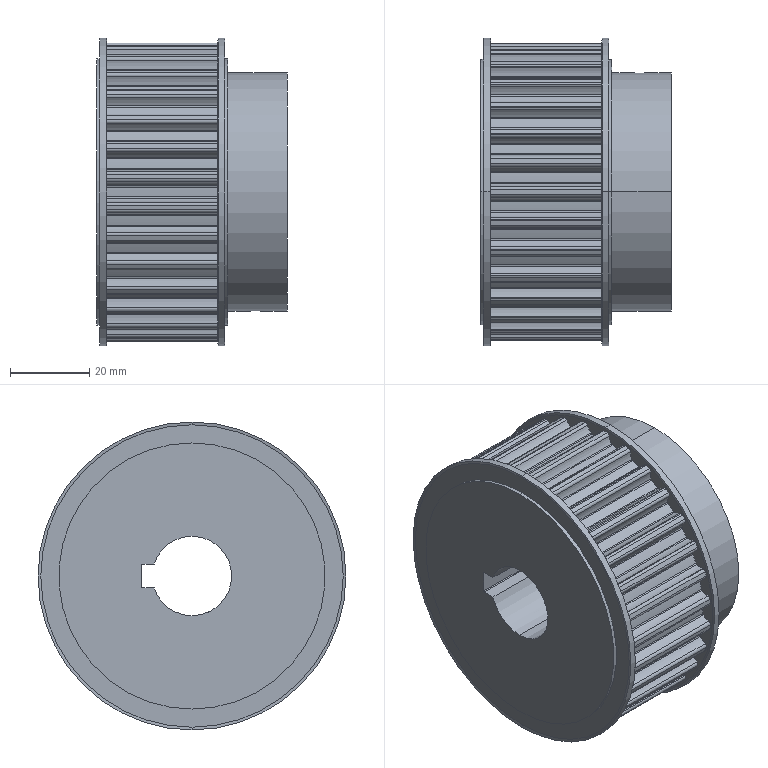Part | STEP file | HTPA30S8M250-B-N20-KC90-FC77.5-TPC5 | 1 solid | 302 faces | box 48 x 77.5 x 77.5 mm | volume 160610 mm3 | cylinder 284 | plane 10 | cone 8 | commonest cylinder face diameters 1.5 x72 0.8 x68 10.6 x64 75.02 x31 69.36 x30 4.134 x4